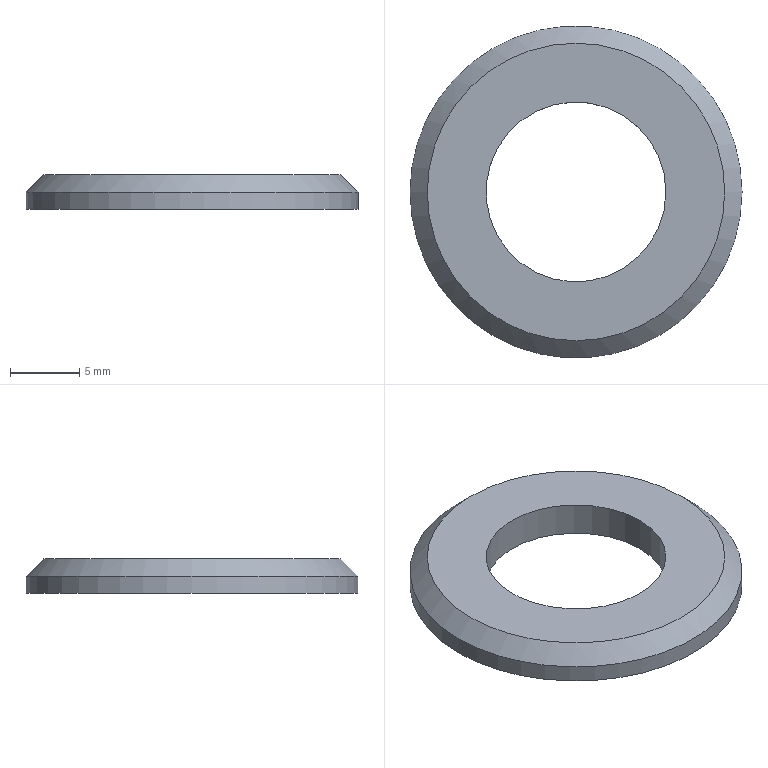Part | NX | features DATUM_CSYS 2, CHAMFER 1, EXTRUDE 1, LINE 1, SKETCH 1 | 1 solid | 5 faces | box 24 x 24 x 2.5 mm | volume 742.283 mm3 | cylinder 2 | plane 2 | cone 1 | commonest cylinder face diameters 13 x1 24 x1
STEP:
#1=CARTESIAN_POINT('',(12.,0.,1.25));
#2=VERTEX_POINT('',#1);
#3=CARTESIAN_POINT('',(0.,0.,1.25));
#4=DIRECTION('',(0.,0.,1.));
#5=DIRECTION('',(1.,0.,0.));
#6=AXIS2_PLACEMENT_3D('',#3,#4,#5);
#7=CIRCLE('',#6,12.);
#8=EDGE_CURVE('',#2,#2,#7,.F.);
#9=ORIENTED_EDGE('',*,*,#8,.T.);
#10=EDGE_LOOP('',(#9));
#11=FACE_BOUND('',#10,.T.);
#12=CARTESIAN_POINT('',(12.,0.,0.));
#13=VERTEX_POINT('',#12);
#14=CARTESIAN_POINT('',(0.,0.,0.));
#15=DIRECTION('',(0.,0.,1.));
#16=DIRECTION('',(1.,0.,0.));
#17=AXIS2_PLACEMENT_3D('',#14,#15,#16);
#18=CIRCLE('',#17,12.);
#19=EDGE_CURVE('',#13,#13,#18,.T.);
#20=ORIENTED_EDGE('',*,*,#19,.T.);
#21=EDGE_LOOP('',(#20));
#22=FACE_BOUND('',#21,.T.);
#23=CARTESIAN_POINT('',(0.,0.,2.5));
#24=DIRECTION('',(0.,0.,-1.));
#25=DIRECTION('',(-1.,0.,0.));
#26=AXIS2_PLACEMENT_3D('',#23,#24,#25);
#27=CYLINDRICAL_SURFACE('',#26,12.);
#28=ADVANCED_FACE('',(#11,#22),#27,.T.);
#29=CARTESIAN_POINT('',(6.5,0.,2.5));
#30=VERTEX_POINT('',#29);
#31=CARTESIAN_POINT('',(0.,0.,2.5));
#32=DIRECTION('',(0.,0.,1.));
#33=DIRECTION('',(1.,0.,0.));
#34=AXIS2_PLACEMENT_3D('',#31,#32,#33);
#35=CIRCLE('',#34,6.5);
#36=EDGE_CURVE('',#30,#30,#35,.T.);
#37=ORIENTED_EDGE('',*,*,#36,.T.);
#38=EDGE_LOOP('',(#37));
#39=FACE_BOUND('',#38,.T.);
#40=CARTESIAN_POINT('',(6.5,0.,0.));
#41=VERTEX_POINT('',#40);
#42=CARTESIAN_POINT('',(0.,0.,0.));
#43=DIRECTION('',(0.,0.,1.));
#44=DIRECTION('',(1.,0.,0.));
#45=AXIS2_PLACEMENT_3D('',#42,#43,#44);
#46=CIRCLE('',#45,6.5);
#47=EDGE_CURVE('',#41,#41,#46,.T.);
#48=ORIENTED_EDGE('',*,*,#47,.F.);
#49=EDGE_LOOP('',(#48));
#50=FACE_BOUND('',#49,.T.);
#51=CARTESIAN_POINT('',(0.,0.,2.5));
#52=DIRECTION('',(0.,0.,-1.));
#53=DIRECTION('',(-1.,0.,0.));
#54=AXIS2_PLACEMENT_3D('',#51,#52,#53);
#55=CYLINDRICAL_SURFACE('',#54,6.5);
#56=ADVANCED_FACE('',(#39,#50),#55,.F.);
#57=CARTESIAN_POINT('',(10.75,0.,2.5));
#58=VERTEX_POINT('',#57);
#59=CARTESIAN_POINT('',(0.,0.,2.5));
#60=DIRECTION('',(0.,0.,1.));
#61=DIRECTION('',(1.,0.,0.));
#62=AXIS2_PLACEMENT_3D('',#59,#60,#61);
#63=CIRCLE('',#62,10.75);
#64=EDGE_CURVE('',#58,#58,#63,.T.);
#65=ORIENTED_EDGE('',*,*,#64,.T.);
#66=EDGE_LOOP('',(#65));
#67=FACE_BOUND('',#66,.T.);
#68=ORIENTED_EDGE('',*,*,#36,.F.);
#69=EDGE_LOOP('',(#68));
#70=FACE_BOUND('',#69,.T.);
#71=CARTESIAN_POINT('',(0.,0.,2.5));
#72=DIRECTION('',(0.,0.,1.));
#73=DIRECTION('',(1.,0.,0.));
#74=AXIS2_PLACEMENT_3D('',#71,#72,#73);
#75=PLANE('',#74);
#76=ADVANCED_FACE('',(#67,#70),#75,.T.);
#77=ORIENTED_EDGE('',*,*,#19,.F.);
#78=EDGE_LOOP('',(#77));
#79=FACE_BOUND('',#78,.T.);
#80=ORIENTED_EDGE('',*,*,#47,.T.);
#81=EDGE_LOOP('',(#80));
#82=FACE_BOUND('',#81,.T.);
#83=CARTESIAN_POINT('',(0.,0.,0.));
#84=DIRECTION('',(0.,0.,1.));
#85=DIRECTION('',(1.,0.,0.));
#86=AXIS2_PLACEMENT_3D('',#83,#84,#85);
#87=PLANE('',#86);
#88=ADVANCED_FACE('',(#79,#82),#87,.F.);
#89=ORIENTED_EDGE('',*,*,#8,.F.);
#90=EDGE_LOOP('',(#89));
#91=FACE_BOUND('',#90,.T.);
#92=ORIENTED_EDGE('',*,*,#64,.F.);
#93=EDGE_LOOP('',(#92));
#94=FACE_BOUND('',#93,.T.);
#95=CARTESIAN_POINT('',(0.,0.,2.5));
#96=DIRECTION('',(0.,0.,-1.));
#97=DIRECTION('',(-1.,0.,0.));
#98=AXIS2_PLACEMENT_3D('',#95,#96,#97);
#99=CONICAL_SURFACE('',#98,10.75,0.7854);
#100=ADVANCED_FACE('',(#91,#94),#99,.T.);
#101=CLOSED_SHELL('',(#28,#56,#76,#88,#100));
#102=MANIFOLD_SOLID_BREP('',#101);
#103=(LENGTH_UNIT()NAMED_UNIT(*)SI_UNIT(.MILLI.,.METRE.));
#104=UNCERTAINTY_MEASURE_WITH_UNIT(LENGTH_MEASURE(0.00001),#103,'','');
#105=(NAMED_UNIT(*)PLANE_ANGLE_UNIT()SI_UNIT($,.RADIAN.));
#106=(NAMED_UNIT(*)SI_UNIT($,.STERADIAN.)SOLID_ANGLE_UNIT());
#107=(GEOMETRIC_REPRESENTATION_CONTEXT(3)GLOBAL_UNCERTAINTY_ASSIGNED_CONTEXT((#104))GLOBAL_UNIT_ASSIGNED_CONTEXT((#103,#105,#106))REPRESENTATION_CONTEXT('',''));
#108=ADVANCED_BREP_SHAPE_REPRESENTATION('',(#102),#107);